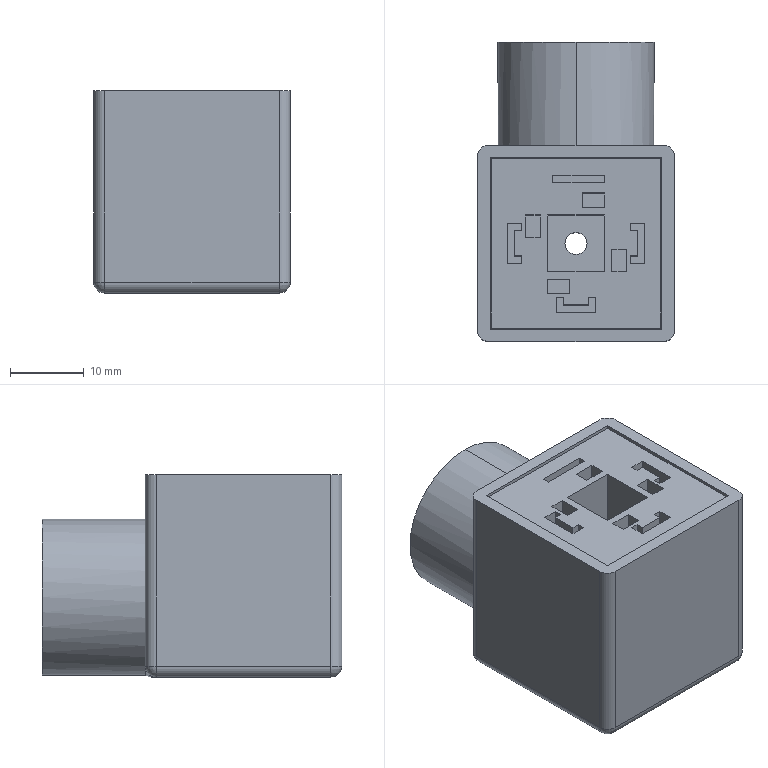Part | STEP file | 1 solid | 123 faces | box 26.7 x 40.7 x 27.46 mm | volume 19718 mm3 | plane 79 | cylinder 35 | sphere 4 | spline 3 | cone 2 | commonest cylinder face diameters 18 x18 3 x11 3.5 x2 8 x2 21.2 x2